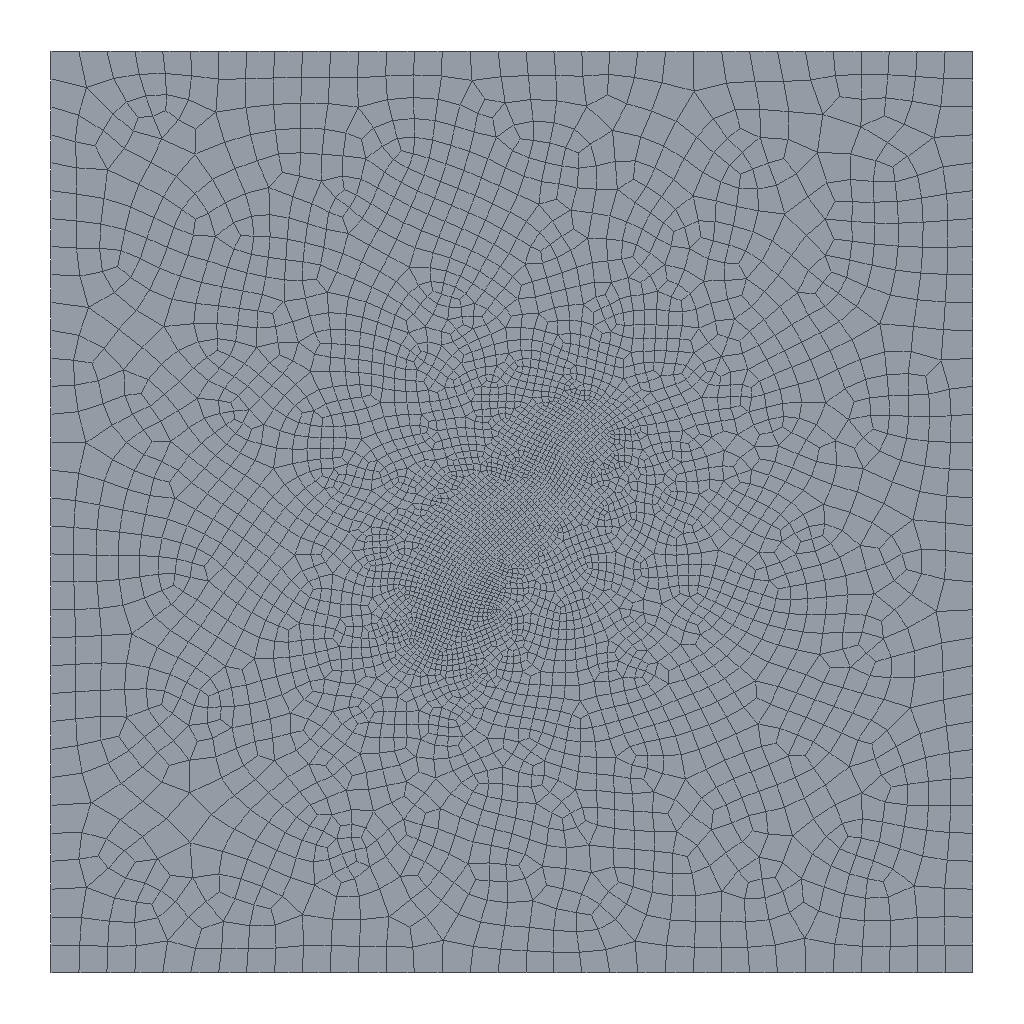Simulation study | abaqus
Set-up summary:
category,name,step,type,value,unit,region
solver,abaqus
solver,version,,,Abaqus/Standard 2020
units,not stated in the deck,,not stated
analysis,deck,,geostatic,geostatic
load_step,Step-1,Step-1,geostatic
load_step,Step-2,Step-2,soils
load_step,requested,,,2
mesh,nodes,,,4874
mesh,elements,,,4734
element_type,CPE4RP,,plane,4659
element_type,COH2D4P,,cohesive,75
load,load commands in deck,,count,1
bc,support commands in deck,,count,4
material,BASE,,in results
material,COH,,in results
check,setup vs results,,match,"per instance, exact: element labels, types and connectivity; labels of the nodes the elements use; coordinates of those nodes at SINGLE_PRECISION in 1 of 1 instance(s)"
Abaqus input file, long lists of numbers shortened:
*Heading
** Job name: Job-5 Model name: Model-1-Copy-Copy
** Generated by: Abaqus/CAE 2020
*Preprint, echo=NO, model=NO, history=NO, contact=NO
**
** PARTS
**
*Part, name=Part-1
*Node
      1,          50.,         -50.
      2,   39.395,  -67.675
** (4872 more lines like these left out)
*Element, type=CPE4RP
   1,  157, 3489, 3446,  156
   2, 3446, 3646,  656, 3573
** (4657 more lines like these left out)
*Element, type=COH2D4P
4660,    2,   48, 4727,    2,    2, 4801
4661,   48,   47, 4728, 4727, 4801, 4802
** (73 more lines like these left out)
*Nset, nset=Set-9, generate
    1,  4800,     1
*Elset, elset=Set-9, generate
    1,  4659,     1
*Elset, elset=CohesiveSeam-4-Elements, generate
 4660,  4734,     1
*Nset, nset=CohesiveSeam-4-TopNodes
    1,    2,    3,   49,   50,   51,   52,   53,   54,   55,   56,   57,   58,   59,   60,   61
   62,   63,   64,   65,   66,   67,   68,   69,   70,   71,   72,   73,   74,   75,   76,   77
** (3 more lines like these left out)
*Nset, nset=CohesiveSeam-4-BottomNodes
    1,    2,    3,    8,    9,   10,   11,   12,   13,   14,   15,   16,   17,   18,   19,   20
   21,   22,   23,   24,   25,   26,   27,   28,   29,   30,   31,   32,   33,   34,   35,   36
** (3 more lines like these left out)
*Nset, nset=CohesiveSeam-4-MidNodes
    2,    3, 4801, 4802, 4803, 4804, 4805, 4806, 4807, 4808, 4809, 4810, 4811, 4812, 4813, 4814
 4815, 4816, 4817, 4818, 4819, 4820, 4821, 4822, 4823, 4824, 4825, 4826, 4827, 4828, 4829, 4830
** (3 more lines like these left out)
*Nset, nset=in
 4842,
*Nset, nset=d
 4841, 4843
*Elset, elset=initial
 4701, 4702
*Elset, elset=__PickedSurf59_S3, internal
  107,  127,  459,  532,  567,  570,  611,  928,  932,  933,  934,  936,  937,  938,  939,  940
  941,  943,  946,  947,  954,  959,  961,  963,  964,  967,  968,  970,  971,  972,  978,  980
** (6 more lines like these left out)
*Elset, elset=__PickedSurf59_S1, internal
  128,  388,  565,  925,  926,  929,  931,  942,  944,  945,  948,  949,  950,  951,  952,  953
  955,  956,  957,  958,  960,  962,  965,  966,  973,  974,  975,  976,  977,  979, 1110, 1121
** (1 more lines like these left out)
*Surface, type=ELEMENT, name=_PickedSurf59, internal
__PickedSurf59_S3, S3
__PickedSurf59_S1, S1
*Elset, elset=_CohesiveSeam-4-TopSurf_S3, internal, generate
 4660,  4734,     1
*Surface, type=ELEMENT, name=CohesiveSeam-4-TopSurf
_CohesiveSeam-4-TopSurf_S3, S3
*Elset, elset=_CohesiveSeam-4-BottomSurf_S1, internal, generate
 4660,  4734,     1
*Surface, type=ELEMENT, name=CohesiveSeam-4-BottomSurf
_CohesiveSeam-4-BottomSurf_S1, S1
** Section: base
*Solid Section, elset=Set-9, material=base
,
** Section: Section-coh
*Cohesive Section, elset=CohesiveSeam-4-Elements, controls=EC-1, material=coh, response=TRACTION SEPARATION
,
*End Part
**
**
** ASSEMBLY
**
*Assembly, name=Assembly
**
*Instance, name=Part-1-1, part=Part-1
*End Instance
**
*Nset, nset=Set-1, instance=Part-1-1
   4,   5,   6,   7,  81,  82,  83,  84,  85,  86,  87,  88,  89,  90,  91,  92
  93,  94,  95,  96,  97,  98,  99, 100, 101, 102, 103, 104, 105, 106, 107, 108
** (3 more lines like these left out)
*Elset, elset=Set-1, instance=Part-1-1
    1,   20,   60,   62,  174,  179,  180,  184,  187,  189,  190,  198,  205,  213,  220,  228
  234,  249,  257,  258,  272,  273,  280,  293,  300,  328,  336,  343,  349,  353,  355,  356
** (3 more lines like these left out)
*Nset, nset=Set-2, instance=Part-1-1
   4,   5,   6,   7, 113, 114, 115, 116, 117, 118, 119, 120, 121, 122, 123, 124
 125, 126, 127, 128, 129, 130, 131, 132, 133, 134, 135, 136, 137, 138, 139, 140
** (3 more lines like these left out)
*Elset, elset=Set-2, instance=Part-1-1
   11,   28,   29,   30,   52,   54,   55,   91,  146,  148,  174,  175,  176,  177,  300,  301
  302,  303,  305,  306,  307,  308,  309,  310,  311,  312,  320,  321,  337,  338,  345,  354
** (3 more lines like these left out)
*Nset, nset=Set-3, instance=Part-1-1, generate
    1,  4800,     1
*Elset, elset=Set-3, instance=Part-1-1, generate
    1,  4659,     1
*Nset, nset=Set-4, instance=Part-1-1, generate
    1,  4800,     1
*Elset, elset=Set-4, instance=Part-1-1, generate
    1,  4659,     1
*Nset, nset=Set-5, instance=Part-1-1
   4,   5,  81,  82,  83,  84,  85,  86,  87,  88,  89,  90,  91,  92,  93,  94
  95,  96,  97,  98,  99, 100, 101, 102, 103, 104, 105, 106, 107, 108, 109, 110
** (1 more lines like these left out)
*Elset, elset=Set-5, instance=Part-1-1
   60,   62,  174,  179,  180,  184,  187,  189,  190,  198,  205,  213,  220,  228,  234,  249
  257,  258,  272,  273,  280,  293,  300, 1035, 1036, 1037, 1038, 3981, 3984, 3987, 4009, 4010
** (1 more lines like these left out)
*Nset, nset=Set-6, instance=Part-1-1
   5,   6, 113, 114, 115, 116, 117, 118, 119, 120, 121, 122, 123, 124, 125, 126
 127, 128, 129, 130, 131, 132, 133, 134, 135, 136, 137, 138, 139, 140, 141, 142
** (1 more lines like these left out)
*Elset, elset=Set-6, instance=Part-1-1
   11,   28,   29,   30,  300,  301,  302,  303,  305,  306,  307,  308,  309,  310,  311,  312
  320,  321,  337,  338,  345,  354,  358, 1039, 1040, 1041, 1042, 1043, 3991, 3994, 4016, 4017
** (1 more lines like these left out)
*Nset, nset=Set-7, instance=Part-1-1
   5,   6, 113, 114, 115, 116, 117, 118, 119, 120, 121, 122, 123, 124, 125, 126
 127, 128, 129, 130, 131, 132, 133, 134, 135, 136, 137, 138, 139, 140, 141, 142
** (1 more lines like these left out)
*Elset, elset=Set-7, instance=Part-1-1
   11,   28,   29,   30,  300,  301,  302,  303,  305,  306,  307,  308,  309,  310,  311,  312
  320,  321,  337,  338,  345,  354,  358, 1039, 1040, 1041, 1042, 1043, 3991, 3994, 4016, 4017
** (1 more lines like these left out)
*Nset, nset=Set-8, instance=Part-1-1
   4,   5,  81,  82,  83,  84,  85,  86,  87,  88,  89,  90,  91,  92,  93,  94
  95,  96,  97,  98,  99, 100, 101, 102, 103, 104, 105, 106, 107, 108, 109, 110
** (1 more lines like these left out)
*Elset, elset=Set-8, instance=Part-1-1
   60,   62,  174,  179,  180,  184,  187,  189,  190,  198,  205,  213,  220,  228,  234,  249
  257,  258,  272,  273,  280,  293,  300, 1035, 1036, 1037, 1038, 3981, 3984, 3987, 4009, 4010
** (1 more lines like these left out)
*End Assembly
**
** ELEMENT CONTROLS
**
*Section Controls, name=EC-1, ELEMENT DELETION=YES
1., 1., 1.
*Amplitude, name=Amp-1
             0.,              0.,             50.,              1.
**
** MATERIALS
**
*Material, name=base
*Elastic
 1.5e+10, 0.25
*Permeability, specific=9800.
 1e-07, 0.2
*Material, name=coh
*Damage Initiation, criterion=MAXS
 1e+06, 5e+06, 5e+06
*Damage Evolution, type=DISPLACEMENT
1.,
*Elastic, type=TRACTION
 1.5e+10, 1.5e+10, 1.5e+10
*Gap Flow
 0.001,
**
** PREDEFINED FIELDS
**
** Name: Predefined Field-1   Type: Void ratio
*Initial Conditions, TYPE=RATIO
Set-3, 0.2
** Name: Predefined Field-2   Type: Stress
*Initial Conditions, type=STRESS
Set-4, -1e+06, -1e+06, -1e+06, 0.,
** ----------------------------------------------------------------
*initial conditions,type=initial gap
part-1-1.initial
**
** STEP: Step-1
**
*Step, name=Step-1, nlgeom=NO, unsymm=YES
*Geostatic
**
** BOUNDARY CONDITIONS
**
** Name: BC-1 Type: 位移/转角
*Boundary
Set-1, 2, 2
** Name: BC-2 Type: 位移/转角
*Boundary
Set-2, 1, 1
**
** OUTPUT REQUESTS
**
*Restart, write, frequency=0
**
** FIELD OUTPUT: F-Output-1
**
*Output, field
*Node Output
CF, PHILSM, POR, PSILSM, RF, U
*Element Output, directions=YES
E, FLUVR, FLVEL, LE, MISES, S, SAT, SDEG, VOIDR
*Contact Output
CSDMG, PFL, PFLA, PTL, PTLA
**
** HISTORY OUTPUT: H-Output-1
**
*Output, history, variable=PRESELECT
*End Step
** ----------------------------------------------------------------
**
** STEP: Step-2
**
*Step, name=Step-2, nlgeom=YES, inc=1000, unsymm=YES
*Soils, consolidation, end=PERIOD, utol=1e+25, creep=none
0.01, 500., 1e-05, 5.,
**
** BOUNDARY CONDITIONS
**
** Name: BC-1 Type: 位移/转角
*Boundary, op=NEW
** Name: BC-2 Type: 位移/转角
*Boundary, op=NEW
** Name: BC-5 Type: 位移/转角
*Boundary, op=NEW
Set-7, 1, 1
** Name: BC-6 Type: 位移/转角
*Boundary, op=NEW
Set-8, 2, 2
**
** LOADS
**
** Name: Load-1   Type: Concentrated pore fluid
*Cflow, amplitude=Amp-1
Part-1-1.in,  , -0.001
**
** CONTROLS
**
*Controls, reset
**
** OUTPUT REQUESTS
**
*Restart, write, frequency=0
**
** FIELD OUTPUT: F-Output-1
**
*Output, field
*Node Output
CF, PHILSM, POR, PSILSM, RF, U
*Element Output, directions=YES
E, FLUVR, FLVEL, LE, MISES, S, SAT, SDEG, VOIDR,pfopen
*Contact Output
CSDMG, PFL, PFLA, PTL, PTLA
**
** HISTORY OUTPUT: H-Output-1
**
*Output, history, variable=PRESELECT
*End Step
Results summary:
result,step,,completed,increments=1 time=1.0/1.0
result,step,,partial,increments=36 time=87.579/500.0
result,analysis,,,"soils, consolidation"
result,last_loadstep,,,2
result,primary field,,,"U, POR"
result,reaction total,,FX,-0.02734,model units
result,reaction total,,FY,-0.009766,model units
result,reaction total,,FZ,0.0,model units